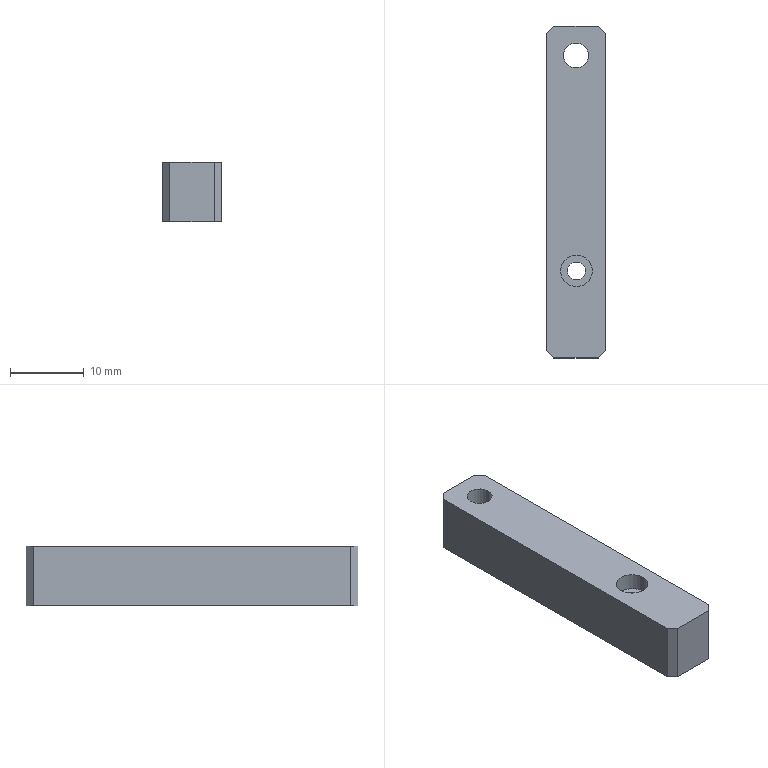Part | SolidWorks | features MirrorStock 1 | 1 solid | 23 faces | box 8 x 45 x 8 mm | volume 2651 mm3 | plane 13 | cylinder 10 | commonest cylinder face diameters 2.4 x2 3.4 x2 4 x2 4.3 x2 6 x2
STEP:
#1=CARTESIAN_POINT('',(-12.431,-38.2,-2.3));
#2=VERTEX_POINT('',#1);
#3=CARTESIAN_POINT('',(-8.131,-38.2,-2.3));
#4=VERTEX_POINT('',#3);
#5=CARTESIAN_POINT('',(-10.281,-38.2,-2.3));
#6=DIRECTION('',(0.,0.,-1.));
#7=DIRECTION('',(-1.,0.,0.));
#8=AXIS2_PLACEMENT_3D('',#5,#6,#7);
#9=CIRCLE('',#8,2.15);
#10=EDGE_CURVE('',#2,#4,#9,.T.);
#11=ORIENTED_EDGE('',*,*,#10,.T.);
#12=CARTESIAN_POINT('',(-8.131,-38.2,0.));
#13=VERTEX_POINT('',#12);
#14=CARTESIAN_POINT('',(-8.131,-38.2,0.));
#15=DIRECTION('',(0.,0.,1.));
#16=VECTOR('',#15,1000.);
#17=LINE('',#14,#16);
#18=EDGE_CURVE('',#4,#13,#17,.T.);
#19=ORIENTED_EDGE('',*,*,#18,.T.);
#20=CARTESIAN_POINT('',(-12.431,-38.2,0.));
#21=VERTEX_POINT('',#20);
#22=CARTESIAN_POINT('',(-10.281,-38.2,0.));
#23=DIRECTION('',(0.,0.,-1.));
#24=DIRECTION('',(-1.,0.,0.));
#25=AXIS2_PLACEMENT_3D('',#22,#23,#24);
#26=CIRCLE('',#25,2.15);
#27=EDGE_CURVE('',#21,#13,#26,.T.);
#28=ORIENTED_EDGE('',*,*,#27,.F.);
#29=CARTESIAN_POINT('',(-12.431,-38.2,0.));
#30=DIRECTION('',(0.,0.,1.));
#31=VECTOR('',#30,1000.);
#32=LINE('',#29,#31);
#33=EDGE_CURVE('',#2,#21,#32,.T.);
#34=ORIENTED_EDGE('',*,*,#33,.F.);
#35=EDGE_LOOP('',(#11,#19,#28,#34));
#36=FACE_OUTER_BOUND('',#35,.T.);
#37=CARTESIAN_POINT('',(-10.281,-38.2,0.));
#38=DIRECTION('',(0.,0.,1.));
#39=DIRECTION('',(-1.,0.,0.));
#40=AXIS2_PLACEMENT_3D('',#37,#38,#39);
#41=CYLINDRICAL_SURFACE('',#40,2.15);
#42=ADVANCED_FACE('',(#36),#41,.F.);
#43=CARTESIAN_POINT('',(-9.081,-38.2,-6.));
#44=VERTEX_POINT('',#43);
#45=CARTESIAN_POINT('',(-11.481,-38.2,-6.));
#46=VERTEX_POINT('',#45);
#47=CARTESIAN_POINT('',(-10.281,-38.2,-6.));
#48=DIRECTION('',(0.,0.,1.));
#49=DIRECTION('',(1.,0.,0.));
#50=AXIS2_PLACEMENT_3D('',#47,#48,#49);
#51=CIRCLE('',#50,1.2);
#52=EDGE_CURVE('',#44,#46,#51,.T.);
#53=ORIENTED_EDGE('',*,*,#52,.F.);
#54=CARTESIAN_POINT('',(-9.081,-38.2,-2.3));
#55=VERTEX_POINT('',#54);
#56=CARTESIAN_POINT('',(-9.081,-38.2,0.));
#57=DIRECTION('',(0.,0.,1.));
#58=VECTOR('',#57,1000.);
#59=LINE('',#56,#58);
#60=EDGE_CURVE('',#44,#55,#59,.T.);
#61=ORIENTED_EDGE('',*,*,#60,.T.);
#62=CARTESIAN_POINT('',(-11.481,-38.2,-2.3));
#63=VERTEX_POINT('',#62);
#64=CARTESIAN_POINT('',(-10.281,-38.2,-2.3));
#65=DIRECTION('',(0.,0.,-1.));
#66=DIRECTION('',(-1.,0.,0.));
#67=AXIS2_PLACEMENT_3D('',#64,#65,#66);
#68=CIRCLE('',#67,1.2);
#69=EDGE_CURVE('',#63,#55,#68,.T.);
#70=ORIENTED_EDGE('',*,*,#69,.F.);
#71=CARTESIAN_POINT('',(-11.481,-38.2,0.));
#72=DIRECTION('',(0.,0.,1.));
#73=VECTOR('',#72,1000.);
#74=LINE('',#71,#73);
#75=EDGE_CURVE('',#46,#63,#74,.T.);
#76=ORIENTED_EDGE('',*,*,#75,.F.);
#77=EDGE_LOOP('',(#53,#61,#70,#76));
#78=FACE_OUTER_BOUND('',#77,.T.);
#79=CARTESIAN_POINT('',(-10.281,-38.2,0.));
#80=DIRECTION('',(0.,0.,1.));
#81=DIRECTION('',(-1.,0.,0.));
#82=AXIS2_PLACEMENT_3D('',#79,#80,#81);
#83=CYLINDRICAL_SURFACE('',#82,1.2);
#84=ADVANCED_FACE('',(#78),#83,.F.);
#85=CARTESIAN_POINT('',(-8.281,-38.2,-6.));
#86=VERTEX_POINT('',#85);
#87=CARTESIAN_POINT('',(-12.281,-38.2,-6.));
#88=VERTEX_POINT('',#87);
#89=CARTESIAN_POINT('',(-10.281,-38.2,-6.));
#90=DIRECTION('',(0.,0.,1.));
#91=DIRECTION('',(1.,0.,0.));
#92=AXIS2_PLACEMENT_3D('',#89,#90,#91);
#93=CIRCLE('',#92,2.);
#94=EDGE_CURVE('',#86,#88,#93,.T.);
#95=ORIENTED_EDGE('',*,*,#94,.T.);
#96=CARTESIAN_POINT('',(-12.281,-38.2,-8.));
#97=VERTEX_POINT('',#96);
#98=CARTESIAN_POINT('',(-12.281,-38.2,-6.));
#99=DIRECTION('',(0.,0.,-1.));
#100=VECTOR('',#99,1000.);
#101=LINE('',#98,#100);
#102=EDGE_CURVE('',#88,#97,#101,.T.);
#103=ORIENTED_EDGE('',*,*,#102,.T.);
#104=CARTESIAN_POINT('',(-8.281,-38.2,-8.));
#105=VERTEX_POINT('',#104);
#106=CARTESIAN_POINT('',(-10.281,-38.2,-8.));
#107=DIRECTION('',(0.,0.,1.));
#108=DIRECTION('',(1.,0.,0.));
#109=AXIS2_PLACEMENT_3D('',#106,#107,#108);
#110=CIRCLE('',#109,2.);
#111=EDGE_CURVE('',#105,#97,#110,.T.);
#112=ORIENTED_EDGE('',*,*,#111,.F.);
#113=CARTESIAN_POINT('',(-8.281,-38.2,-6.));
#114=DIRECTION('',(0.,0.,-1.));
#115=VECTOR('',#114,1000.);
#116=LINE('',#113,#115);
#117=EDGE_CURVE('',#86,#105,#116,.T.);
#118=ORIENTED_EDGE('',*,*,#117,.F.);
#119=EDGE_LOOP('',(#95,#103,#112,#118));
#120=FACE_OUTER_BOUND('',#119,.T.);
#121=CARTESIAN_POINT('',(-10.281,-38.2,-6.));
#122=DIRECTION('',(0.,0.,-1.));
#123=DIRECTION('',(1.,0.,0.));
#124=AXIS2_PLACEMENT_3D('',#121,#122,#123);
#125=CYLINDRICAL_SURFACE('',#124,2.);
#126=ADVANCED_FACE('',(#120),#125,.F.);
#127=CARTESIAN_POINT('',(-7.345,-9.,-4.6));
#128=VERTEX_POINT('',#127);
#129=CARTESIAN_POINT('',(-13.345,-9.,-4.6));
#130=VERTEX_POINT('',#129);
#131=CARTESIAN_POINT('',(-10.345,-9.,-4.6));
#132=DIRECTION('',(0.,0.,1.));
#133=DIRECTION('',(1.,0.,0.));
#134=AXIS2_PLACEMENT_3D('',#131,#132,#133);
#135=CIRCLE('',#134,3.);
#136=EDGE_CURVE('',#128,#130,#135,.T.);
#137=ORIENTED_EDGE('',*,*,#136,.T.);
#138=CARTESIAN_POINT('',(-13.345,-9.,-8.));
#139=VERTEX_POINT('',#138);
#140=CARTESIAN_POINT('',(-13.345,-9.,-8.));
#141=DIRECTION('',(0.,0.,-1.));
#142=VECTOR('',#141,1000.);
#143=LINE('',#140,#142);
#144=EDGE_CURVE('',#130,#139,#143,.T.);
#145=ORIENTED_EDGE('',*,*,#144,.T.);
#146=CARTESIAN_POINT('',(-7.345,-9.,-8.));
#147=VERTEX_POINT('',#146);
#148=CARTESIAN_POINT('',(-10.345,-9.,-8.));
#149=DIRECTION('',(0.,0.,1.));
#150=DIRECTION('',(1.,0.,0.));
#151=AXIS2_PLACEMENT_3D('',#148,#149,#150);
#152=CIRCLE('',#151,3.);
#153=EDGE_CURVE('',#147,#139,#152,.T.);
#154=ORIENTED_EDGE('',*,*,#153,.F.);
#155=CARTESIAN_POINT('',(-7.345,-9.,-8.));
#156=DIRECTION('',(0.,0.,-1.));
#157=VECTOR('',#156,1000.);
#158=LINE('',#155,#157);
#159=EDGE_CURVE('',#128,#147,#158,.T.);
#160=ORIENTED_EDGE('',*,*,#159,.F.);
#161=EDGE_LOOP('',(#137,#145,#154,#160));
#162=FACE_OUTER_BOUND('',#161,.T.);
#163=CARTESIAN_POINT('',(-10.345,-9.,-8.));
#164=DIRECTION('',(0.,0.,-1.));
#165=DIRECTION('',(1.,0.,0.));
#166=AXIS2_PLACEMENT_3D('',#163,#164,#165);
#167=CYLINDRICAL_SURFACE('',#166,3.);
#168=ADVANCED_FACE('',(#162),#167,.F.);
#169=CARTESIAN_POINT('',(-8.645,-9.,0.));
#170=VERTEX_POINT('',#169);
#171=CARTESIAN_POINT('',(-12.045,-9.,0.));
#172=VERTEX_POINT('',#171);
#173=CARTESIAN_POINT('',(-10.345,-9.,0.));
#174=DIRECTION('',(0.,0.,1.));
#175=DIRECTION('',(1.,0.,0.));
#176=AXIS2_PLACEMENT_3D('',#173,#174,#175);
#177=CIRCLE('',#176,1.7);
#178=EDGE_CURVE('',#170,#172,#177,.T.);
#179=ORIENTED_EDGE('',*,*,#178,.T.);
#180=CARTESIAN_POINT('',(-12.045,-9.,-4.6));
#181=VERTEX_POINT('',#180);
#182=CARTESIAN_POINT('',(-12.045,-9.,-8.));
#183=DIRECTION('',(0.,0.,-1.));
#184=VECTOR('',#183,1000.);
#185=LINE('',#182,#184);
#186=EDGE_CURVE('',#172,#181,#185,.T.);
#187=ORIENTED_EDGE('',*,*,#186,.T.);
#188=CARTESIAN_POINT('',(-8.645,-9.,-4.6));
#189=VERTEX_POINT('',#188);
#190=CARTESIAN_POINT('',(-10.345,-9.,-4.6));
#191=DIRECTION('',(0.,0.,1.));
#192=DIRECTION('',(1.,0.,0.));
#193=AXIS2_PLACEMENT_3D('',#190,#191,#192);
#194=CIRCLE('',#193,1.7);
#195=EDGE_CURVE('',#189,#181,#194,.T.);
#196=ORIENTED_EDGE('',*,*,#195,.F.);
#197=CARTESIAN_POINT('',(-8.645,-9.,-8.));
#198=DIRECTION('',(0.,0.,-1.));
#199=VECTOR('',#198,1000.);
#200=LINE('',#197,#199);
#201=EDGE_CURVE('',#170,#189,#200,.T.);
#202=ORIENTED_EDGE('',*,*,#201,.F.);
#203=EDGE_LOOP('',(#179,#187,#196,#202));
#204=FACE_OUTER_BOUND('',#203,.T.);
#205=CARTESIAN_POINT('',(-10.345,-9.,-8.));
#206=DIRECTION('',(0.,0.,-1.));
#207=DIRECTION('',(1.,0.,0.));
#208=AXIS2_PLACEMENT_3D('',#205,#206,#207);
#209=CYLINDRICAL_SURFACE('',#208,1.7);
#210=ADVANCED_FACE('',(#204),#209,.F.);
#211=CARTESIAN_POINT('',(-13.345,-5.,-8.));
#212=VERTEX_POINT('',#211);
#213=CARTESIAN_POINT('',(-7.345,-5.,-8.));
#214=VERTEX_POINT('',#213);
#215=CARTESIAN_POINT('',(-14.345,-5.,-8.));
#216=DIRECTION('',(1.,0.,0.));
#217=VECTOR('',#216,1000.);
#218=LINE('',#215,#217);
#219=EDGE_CURVE('',#212,#214,#218,.T.);
#220=ORIENTED_EDGE('',*,*,#219,.F.);
#221=CARTESIAN_POINT('',(-13.345,-5.,0.));
#222=VERTEX_POINT('',#221);
#223=CARTESIAN_POINT('',(-13.345,-5.,-8.));
#224=DIRECTION('',(0.,0.,-1.));
#225=VECTOR('',#224,1000.);
#226=LINE('',#223,#225);
#227=EDGE_CURVE('',#222,#212,#226,.T.);
#228=ORIENTED_EDGE('',*,*,#227,.F.);
#229=CARTESIAN_POINT('',(-7.345,-5.,0.));
#230=VERTEX_POINT('',#229);
#231=CARTESIAN_POINT('',(-14.345,-5.,0.));
#232=DIRECTION('',(1.,0.,0.));
#233=VECTOR('',#232,1000.);
#234=LINE('',#231,#233);
#235=EDGE_CURVE('',#222,#230,#234,.T.);
#236=ORIENTED_EDGE('',*,*,#235,.T.);
#237=CARTESIAN_POINT('',(-7.345,-5.,-8.));
#238=DIRECTION('',(0.,0.,1.));
#239=VECTOR('',#238,1000.);
#240=LINE('',#237,#239);
#241=EDGE_CURVE('',#214,#230,#240,.T.);
#242=ORIENTED_EDGE('',*,*,#241,.F.);
#243=EDGE_LOOP('',(#220,#228,#236,#242));
#244=FACE_OUTER_BOUND('',#243,.T.);
#245=CARTESIAN_POINT('',(-14.345,-5.,-8.));
#246=DIRECTION('',(0.,1.,0.));
#247=DIRECTION('',(0.,0.,-1.));
#248=AXIS2_PLACEMENT_3D('',#245,#246,#247);
#249=PLANE('',#248);
#250=ADVANCED_FACE('',(#244),#249,.T.);
#251=CARTESIAN_POINT('',(-14.345,-6.,0.));
#252=VERTEX_POINT('',#251);
#253=CARTESIAN_POINT('',(-14.345,-49.,0.));
#254=VERTEX_POINT('',#253);
#255=CARTESIAN_POINT('',(-14.345,-5.,0.));
#256=DIRECTION('',(0.,-1.,0.));
#257=VECTOR('',#256,1000.);
#258=LINE('',#255,#257);
#259=EDGE_CURVE('',#252,#254,#258,.T.);
#260=ORIENTED_EDGE('',*,*,#259,.F.);
#261=CARTESIAN_POINT('',(-14.345,-6.,-8.));
#262=VERTEX_POINT('',#261);
#263=CARTESIAN_POINT('',(-14.345,-6.,0.));
#264=DIRECTION('',(0.,0.,1.));
#265=VECTOR('',#264,1000.);
#266=LINE('',#263,#265);
#267=EDGE_CURVE('',#262,#252,#266,.T.);
#268=ORIENTED_EDGE('',*,*,#267,.F.);
#269=CARTESIAN_POINT('',(-14.345,-49.,-8.));
#270=VERTEX_POINT('',#269);
#271=CARTESIAN_POINT('',(-14.345,-5.,-8.));
#272=DIRECTION('',(0.,-1.,0.));
#273=VECTOR('',#272,1000.);
#274=LINE('',#271,#273);
#275=EDGE_CURVE('',#262,#270,#274,.T.);
#276=ORIENTED_EDGE('',*,*,#275,.T.);
#277=CARTESIAN_POINT('',(-14.345,-49.,-8.));
#278=DIRECTION('',(0.,0.,-1.));
#279=VECTOR('',#278,1000.);
#280=LINE('',#277,#279);
#281=EDGE_CURVE('',#254,#270,#280,.T.);
#282=ORIENTED_EDGE('',*,*,#281,.F.);
#283=EDGE_LOOP('',(#260,#268,#276,#282));
#284=FACE_OUTER_BOUND('',#283,.T.);
#285=CARTESIAN_POINT('',(-14.345,-5.,-8.));
#286=DIRECTION('',(1.,0.,0.));
#287=DIRECTION('',(0.,1.,0.));
#288=AXIS2_PLACEMENT_3D('',#285,#286,#287);
#289=PLANE('',#288);
#290=ADVANCED_FACE('',(#284),#289,.F.);
#291=CARTESIAN_POINT('',(-13.345,-50.,0.));
#292=VERTEX_POINT('',#291);
#293=CARTESIAN_POINT('',(-7.345,-50.,0.));
#294=VERTEX_POINT('',#293);
#295=CARTESIAN_POINT('',(-14.345,-50.,0.));
#296=DIRECTION('',(1.,0.,0.));
#297=VECTOR('',#296,1000.);
#298=LINE('',#295,#297);
#299=EDGE_CURVE('',#292,#294,#298,.T.);
#300=ORIENTED_EDGE('',*,*,#299,.F.);
#301=CARTESIAN_POINT('',(-13.345,-50.,-8.));
#302=VERTEX_POINT('',#301);
#303=CARTESIAN_POINT('',(-13.345,-50.,-8.));
#304=DIRECTION('',(0.,0.,1.));
#305=VECTOR('',#304,1000.);
#306=LINE('',#303,#305);
#307=EDGE_CURVE('',#302,#292,#306,.T.);
#308=ORIENTED_EDGE('',*,*,#307,.F.);
#309=CARTESIAN_POINT('',(-7.345,-50.,-8.));
#310=VERTEX_POINT('',#309);
#311=CARTESIAN_POINT('',(-14.345,-50.,-8.));
#312=DIRECTION('',(1.,0.,0.));
#313=VECTOR('',#312,1000.);
#314=LINE('',#311,#313);
#315=EDGE_CURVE('',#302,#310,#314,.T.);
#316=ORIENTED_EDGE('',*,*,#315,.T.);
#317=CARTESIAN_POINT('',(-7.345,-50.,-8.));
#318=DIRECTION('',(0.,0.,-1.));
#319=VECTOR('',#318,1000.);
#320=LINE('',#317,#319);
#321=EDGE_CURVE('',#294,#310,#320,.T.);
#322=ORIENTED_EDGE('',*,*,#321,.F.);
#323=EDGE_LOOP('',(#300,#308,#316,#322));
#324=FACE_OUTER_BOUND('',#323,.T.);
#325=CARTESIAN_POINT('',(-14.345,-50.,-8.));
#326=DIRECTION('',(0.,1.,0.));
#327=DIRECTION('',(0.,0.,-1.));
#328=AXIS2_PLACEMENT_3D('',#325,#326,#327);
#329=PLANE('',#328);
#330=ADVANCED_FACE('',(#324),#329,.F.);
#331=CARTESIAN_POINT('',(-6.345,-6.,-8.));
#332=VERTEX_POINT('',#331);
#333=CARTESIAN_POINT('',(-6.345,-49.,-8.));
#334=VERTEX_POINT('',#333);
#335=CARTESIAN_POINT('',(-6.345,-5.,-8.));
#336=DIRECTION('',(0.,-1.,0.));
#337=VECTOR('',#336,1000.);
#338=LINE('',#335,#337);
#339=EDGE_CURVE('',#332,#334,#338,.T.);
#340=ORIENTED_EDGE('',*,*,#339,.F.);
#341=CARTESIAN_POINT('',(-6.345,-6.,0.));
#342=VERTEX_POINT('',#341);
#343=CARTESIAN_POINT('',(-6.345,-6.,-8.));
#344=DIRECTION('',(0.,0.,-1.));
#345=VECTOR('',#344,1000.);
#346=LINE('',#343,#345);
#347=EDGE_CURVE('',#342,#332,#346,.T.);
#348=ORIENTED_EDGE('',*,*,#347,.F.);
#349=CARTESIAN_POINT('',(-6.345,-49.,0.));
#350=VERTEX_POINT('',#349);
#351=CARTESIAN_POINT('',(-6.345,-5.,0.));
#352=DIRECTION('',(0.,-1.,0.));
#353=VECTOR('',#352,1000.);
#354=LINE('',#351,#353);
#355=EDGE_CURVE('',#342,#350,#354,.T.);
#356=ORIENTED_EDGE('',*,*,#355,.T.);
#357=CARTESIAN_POINT('',(-6.345,-49.,0.));
#358=DIRECTION('',(0.,0.,1.));
#359=VECTOR('',#358,1000.);
#360=LINE('',#357,#359);
#361=EDGE_CURVE('',#334,#350,#360,.T.);
#362=ORIENTED_EDGE('',*,*,#361,.F.);
#363=EDGE_LOOP('',(#340,#348,#356,#362));
#364=FACE_OUTER_BOUND('',#363,.T.);
#365=CARTESIAN_POINT('',(-6.345,-5.,-8.));
#366=DIRECTION('',(1.,0.,0.));
#367=DIRECTION('',(0.,1.,0.));
#368=AXIS2_PLACEMENT_3D('',#365,#366,#367);
#369=PLANE('',#368);
#370=ADVANCED_FACE('',(#364),#369,.T.);
#371=ORIENTED_EDGE('',*,*,#111,.T.);
#372=CARTESIAN_POINT('',(-10.281,-38.2,-8.));
#373=DIRECTION('',(0.,0.,1.));
#374=DIRECTION('',(1.,0.,0.));
#375=AXIS2_PLACEMENT_3D('',#372,#373,#374);
#376=CIRCLE('',#375,2.);
#377=EDGE_CURVE('',#97,#105,#376,.T.);
#378=ORIENTED_EDGE('',*,*,#377,.T.);
#379=EDGE_LOOP('',(#371,#378));
#380=FACE_BOUND('',#379,.T.);
#381=ORIENTED_EDGE('',*,*,#153,.T.);
#382=CARTESIAN_POINT('',(-10.345,-9.,-8.));
#383=DIRECTION('',(0.,0.,1.));
#384=DIRECTION('',(1.,0.,0.));
#385=AXIS2_PLACEMENT_3D('',#382,#383,#384);
#386=CIRCLE('',#385,3.);
#387=EDGE_CURVE('',#139,#147,#386,.T.);
#388=ORIENTED_EDGE('',*,*,#387,.T.);
#389=EDGE_LOOP('',(#381,#388));
#390=FACE_BOUND('',#389,.T.);
#391=ORIENTED_EDGE('',*,*,#315,.F.);
#392=CARTESIAN_POINT('',(-13.345,-50.,-8.));
#393=DIRECTION('',(0.7071,-0.7071,0.));
#394=VECTOR('',#393,1000.);
#395=LINE('',#392,#394);
#396=EDGE_CURVE('',#270,#302,#395,.T.);
#397=ORIENTED_EDGE('',*,*,#396,.F.);
#398=ORIENTED_EDGE('',*,*,#275,.F.);
#399=CARTESIAN_POINT('',(-14.345,-6.,-8.));
#400=DIRECTION('',(-0.7071,-0.7071,0.));
#401=VECTOR('',#400,1000.);
#402=LINE('',#399,#401);
#403=EDGE_CURVE('',#212,#262,#402,.T.);
#404=ORIENTED_EDGE('',*,*,#403,.F.);
#405=ORIENTED_EDGE('',*,*,#219,.T.);
#406=CARTESIAN_POINT('',(-7.345,-5.,-8.));
#407=DIRECTION('',(-0.7071,0.7071,0.));
#408=VECTOR('',#407,1000.);
#409=LINE('',#406,#408);
#410=EDGE_CURVE('',#332,#214,#409,.T.);
#411=ORIENTED_EDGE('',*,*,#410,.F.);
#412=ORIENTED_EDGE('',*,*,#339,.T.);
#413=CARTESIAN_POINT('',(-6.345,-49.,-8.));
#414=DIRECTION('',(0.7071,0.7071,0.));
#415=VECTOR('',#414,1000.);
#416=LINE('',#413,#415);
#417=EDGE_CURVE('',#310,#334,#416,.T.);
#418=ORIENTED_EDGE('',*,*,#417,.F.);
#419=EDGE_LOOP('',(#391,#397,#398,#404,#405,#411,#412,#418));
#420=FACE_OUTER_BOUND('',#419,.T.);
#421=CARTESIAN_POINT('',(0.,0.,-8.));
#422=DIRECTION('',(0.,0.,1.));
#423=DIRECTION('',(-1.,0.,0.));
#424=AXIS2_PLACEMENT_3D('',#421,#422,#423);
#425=PLANE('',#424);
#426=ADVANCED_FACE('',(#380,#390,#420),#425,.F.);
#427=ORIENTED_EDGE('',*,*,#27,.T.);
#428=CARTESIAN_POINT('',(-10.281,-38.2,0.));
#429=DIRECTION('',(0.,0.,-1.));
#430=DIRECTION('',(-1.,0.,0.));
#431=AXIS2_PLACEMENT_3D('',#428,#429,#430);
#432=CIRCLE('',#431,2.15);
#433=EDGE_CURVE('',#13,#21,#432,.T.);
#434=ORIENTED_EDGE('',*,*,#433,.T.);
#435=EDGE_LOOP('',(#427,#434));
#436=FACE_BOUND('',#435,.T.);
#437=ORIENTED_EDGE('',*,*,#178,.F.);
#438=CARTESIAN_POINT('',(-10.345,-9.,0.));
#439=DIRECTION('',(0.,0.,1.));
#440=DIRECTION('',(1.,0.,0.));
#441=AXIS2_PLACEMENT_3D('',#438,#439,#440);
#442=CIRCLE('',#441,1.7);
#443=EDGE_CURVE('',#172,#170,#442,.T.);
#444=ORIENTED_EDGE('',*,*,#443,.F.);
#445=EDGE_LOOP('',(#437,#444));
#446=FACE_BOUND('',#445,.T.);
#447=ORIENTED_EDGE('',*,*,#355,.F.);
#448=CARTESIAN_POINT('',(-6.172,-6.172,0.));
#449=DIRECTION('',(0.7071,-0.7071,0.));
#450=VECTOR('',#449,1000.);
#451=LINE('',#448,#450);
#452=EDGE_CURVE('',#230,#342,#451,.T.);
#453=ORIENTED_EDGE('',*,*,#452,.F.);
#454=ORIENTED_EDGE('',*,*,#235,.F.);
#455=CARTESIAN_POINT('',(-4.172,4.172,0.));
#456=DIRECTION('',(0.7071,0.7071,0.));
#457=VECTOR('',#456,1000.);
#458=LINE('',#455,#457);
#459=EDGE_CURVE('',#252,#222,#458,.T.);
#460=ORIENTED_EDGE('',*,*,#459,.F.);
#461=ORIENTED_EDGE('',*,*,#259,.T.);
#462=CARTESIAN_POINT('',(-31.672,-31.672,0.));
#463=DIRECTION('',(-0.7071,0.7071,0.));
#464=VECTOR('',#463,1000.);
#465=LINE('',#462,#464);
#466=EDGE_CURVE('',#292,#254,#465,.T.);
#467=ORIENTED_EDGE('',*,*,#466,.F.);
#468=ORIENTED_EDGE('',*,*,#299,.T.);
#469=CARTESIAN_POINT('',(21.328,-21.328,0.));
#470=DIRECTION('',(-0.7071,-0.7071,0.));
#471=VECTOR('',#470,1000.);
#472=LINE('',#469,#471);
#473=EDGE_CURVE('',#350,#294,#472,.T.);
#474=ORIENTED_EDGE('',*,*,#473,.F.);
#475=EDGE_LOOP('',(#447,#453,#454,#460,#461,#467,#468,#474));
#476=FACE_OUTER_BOUND('',#475,.T.);
#477=CARTESIAN_POINT('',(0.,0.,0.));
#478=DIRECTION('',(0.,0.,1.));
#479=DIRECTION('',(-1.,0.,0.));
#480=AXIS2_PLACEMENT_3D('',#477,#478,#479);
#481=PLANE('',#480);
#482=ADVANCED_FACE('',(#436,#446,#476),#481,.T.);
#483=ORIENTED_EDGE('',*,*,#186,.F.);
#484=ORIENTED_EDGE('',*,*,#443,.T.);
#485=ORIENTED_EDGE('',*,*,#201,.T.);
#486=CARTESIAN_POINT('',(-10.345,-9.,-4.6));
#487=DIRECTION('',(0.,0.,1.));
#488=DIRECTION('',(1.,0.,0.));
#489=AXIS2_PLACEMENT_3D('',#486,#487,#488);
#490=CIRCLE('',#489,1.7);
#491=EDGE_CURVE('',#181,#189,#490,.T.);
#492=ORIENTED_EDGE('',*,*,#491,.F.);
#493=EDGE_LOOP('',(#483,#484,#485,#492));
#494=FACE_OUTER_BOUND('',#493,.T.);
#495=CARTESIAN_POINT('',(-10.345,-9.,-8.));
#496=DIRECTION('',(0.,0.,-1.));
#497=DIRECTION('',(1.,0.,0.));
#498=AXIS2_PLACEMENT_3D('',#495,#496,#497);
#499=CYLINDRICAL_SURFACE('',#498,1.7);
#500=ADVANCED_FACE('',(#494),#499,.F.);
#501=ORIENTED_EDGE('',*,*,#195,.T.);
#502=ORIENTED_EDGE('',*,*,#491,.T.);
#503=EDGE_LOOP('',(#501,#502));
#504=FACE_BOUND('',#503,.T.);
#505=ORIENTED_EDGE('',*,*,#136,.F.);
#506=CARTESIAN_POINT('',(-10.345,-9.,-4.6));
#507=DIRECTION('',(0.,0.,1.));
#508=DIRECTION('',(1.,0.,0.));
#509=AXIS2_PLACEMENT_3D('',#506,#507,#508);
#510=CIRCLE('',#509,3.);
#511=EDGE_CURVE('',#130,#128,#510,.T.);
#512=ORIENTED_EDGE('',*,*,#511,.F.);
#513=EDGE_LOOP('',(#505,#512));
#514=FACE_OUTER_BOUND('',#513,.T.);
#515=CARTESIAN_POINT('',(-8.645,-9.,-4.6));
#516=DIRECTION('',(0.,0.,1.));
#517=DIRECTION('',(-1.,0.,0.));
#518=AXIS2_PLACEMENT_3D('',#515,#516,#517);
#519=PLANE('',#518);
#520=ADVANCED_FACE('',(#504,#514),#519,.F.);
#521=ORIENTED_EDGE('',*,*,#144,.F.);
#522=ORIENTED_EDGE('',*,*,#511,.T.);
#523=ORIENTED_EDGE('',*,*,#159,.T.);
#524=ORIENTED_EDGE('',*,*,#387,.F.);
#525=EDGE_LOOP('',(#521,#522,#523,#524));
#526=FACE_OUTER_BOUND('',#525,.T.);
#527=CARTESIAN_POINT('',(-10.345,-9.,-8.));
#528=DIRECTION('',(0.,0.,-1.));
#529=DIRECTION('',(1.,0.,0.));
#530=AXIS2_PLACEMENT_3D('',#527,#528,#529);
#531=CYLINDRICAL_SURFACE('',#530,3.);
#532=ADVANCED_FACE('',(#526),#531,.F.);
#533=ORIENTED_EDGE('',*,*,#102,.F.);
#534=CARTESIAN_POINT('',(-10.281,-38.2,-6.));
#535=DIRECTION('',(0.,0.,1.));
#536=DIRECTION('',(1.,0.,0.));
#537=AXIS2_PLACEMENT_3D('',#534,#535,#536);
#538=CIRCLE('',#537,2.);
#539=EDGE_CURVE('',#88,#86,#538,.T.);
#540=ORIENTED_EDGE('',*,*,#539,.T.);
#541=ORIENTED_EDGE('',*,*,#117,.T.);
#542=ORIENTED_EDGE('',*,*,#377,.F.);
#543=EDGE_LOOP('',(#533,#540,#541,#542));
#544=FACE_OUTER_BOUND('',#543,.T.);
#545=CARTESIAN_POINT('',(-10.281,-38.2,-6.));
#546=DIRECTION('',(0.,0.,-1.));
#547=DIRECTION('',(1.,0.,0.));
#548=AXIS2_PLACEMENT_3D('',#545,#546,#547);
#549=CYLINDRICAL_SURFACE('',#548,2.);
#550=ADVANCED_FACE('',(#544),#549,.F.);
#551=CARTESIAN_POINT('',(-10.281,-38.2,-6.));
#552=DIRECTION('',(0.,0.,1.));
#553=DIRECTION('',(1.,0.,0.));
#554=AXIS2_PLACEMENT_3D('',#551,#552,#553);
#555=CIRCLE('',#554,1.2);
#556=EDGE_CURVE('',#46,#44,#555,.T.);
#557=ORIENTED_EDGE('',*,*,#556,.T.);
#558=ORIENTED_EDGE('',*,*,#52,.T.);
#559=EDGE_LOOP('',(#557,#558));
#560=FACE_BOUND('',#559,.T.);
#561=ORIENTED_EDGE('',*,*,#94,.F.);
#562=ORIENTED_EDGE('',*,*,#539,.F.);
#563=EDGE_LOOP('',(#561,#562));
#564=FACE_OUTER_BOUND('',#563,.T.);
#565=CARTESIAN_POINT('',(-10.281,-38.2,-6.));
#566=DIRECTION('',(0.,0.,-1.));
#567=DIRECTION('',(1.,0.,0.));
#568=AXIS2_PLACEMENT_3D('',#565,#566,#567);
#569=PLANE('',#568);
#570=ADVANCED_FACE('',(#560,#564),#569,.T.);
#571=ORIENTED_EDGE('',*,*,#60,.F.);
#572=ORIENTED_EDGE('',*,*,#556,.F.);
#573=ORIENTED_EDGE('',*,*,#75,.T.);
#574=CARTESIAN_POINT('',(-10.281,-38.2,-2.3));
#575=DIRECTION('',(0.,0.,-1.));
#576=DIRECTION('',(-1.,0.,0.));
#577=AXIS2_PLACEMENT_3D('',#574,#575,#576);
#578=CIRCLE('',#577,1.2);
#579=EDGE_CURVE('',#55,#63,#578,.T.);
#580=ORIENTED_EDGE('',*,*,#579,.F.);
#581=EDGE_LOOP('',(#571,#572,#573,#580));
#582=FACE_OUTER_BOUND('',#581,.T.);
#583=CARTESIAN_POINT('',(-10.281,-38.2,0.));
#584=DIRECTION('',(0.,0.,1.));
#585=DIRECTION('',(-1.,0.,0.));
#586=AXIS2_PLACEMENT_3D('',#583,#584,#585);
#587=CYLINDRICAL_SURFACE('',#586,1.2);
#588=ADVANCED_FACE('',(#582),#587,.F.);
#589=ORIENTED_EDGE('',*,*,#69,.T.);
#590=ORIENTED_EDGE('',*,*,#579,.T.);
#591=EDGE_LOOP('',(#589,#590));
#592=FACE_BOUND('',#591,.T.);
#593=ORIENTED_EDGE('',*,*,#10,.F.);
#594=CARTESIAN_POINT('',(-10.281,-38.2,-2.3));
#595=DIRECTION('',(0.,0.,-1.));
#596=DIRECTION('',(-1.,0.,0.));
#597=AXIS2_PLACEMENT_3D('',#594,#595,#596);
#598=CIRCLE('',#597,2.15);
#599=EDGE_CURVE('',#4,#2,#598,.T.);
#600=ORIENTED_EDGE('',*,*,#599,.F.);
#601=EDGE_LOOP('',(#593,#600));
#602=FACE_OUTER_BOUND('',#601,.T.);
#603=CARTESIAN_POINT('',(-9.081,-38.2,-2.3));
#604=DIRECTION('',(0.,0.,-1.));
#605=DIRECTION('',(1.,0.,0.));
#606=AXIS2_PLACEMENT_3D('',#603,#604,#605);
#607=PLANE('',#606);
#608=ADVANCED_FACE('',(#592,#602),#607,.F.);
#609=ORIENTED_EDGE('',*,*,#18,.F.);
#610=ORIENTED_EDGE('',*,*,#599,.T.);
#611=ORIENTED_EDGE('',*,*,#33,.T.);
#612=ORIENTED_EDGE('',*,*,#433,.F.);
#613=EDGE_LOOP('',(#609,#610,#611,#612));
#614=FACE_OUTER_BOUND('',#613,.T.);
#615=CARTESIAN_POINT('',(-10.281,-38.2,0.));
#616=DIRECTION('',(0.,0.,1.));
#617=DIRECTION('',(-1.,0.,0.));
#618=AXIS2_PLACEMENT_3D('',#615,#616,#617);
#619=CYLINDRICAL_SURFACE('',#618,2.15);
#620=ADVANCED_FACE('',(#614),#619,.F.);
#621=ORIENTED_EDGE('',*,*,#417,.T.);
#622=ORIENTED_EDGE('',*,*,#361,.T.);
#623=ORIENTED_EDGE('',*,*,#473,.T.);
#624=ORIENTED_EDGE('',*,*,#321,.T.);
#625=EDGE_LOOP('',(#621,#622,#623,#624));
#626=FACE_OUTER_BOUND('',#625,.T.);
#627=CARTESIAN_POINT('',(-6.345,-49.,-8.));
#628=DIRECTION('',(0.7071,-0.7071,0.));
#629=DIRECTION('',(0.,0.,-1.));
#630=AXIS2_PLACEMENT_3D('',#627,#628,#629);
#631=PLANE('',#630);
#632=ADVANCED_FACE('',(#626),#631,.T.);
#633=ORIENTED_EDGE('',*,*,#396,.T.);
#634=ORIENTED_EDGE('',*,*,#307,.T.);
#635=ORIENTED_EDGE('',*,*,#466,.T.);
#636=ORIENTED_EDGE('',*,*,#281,.T.);
#637=EDGE_LOOP('',(#633,#634,#635,#636));
#638=FACE_OUTER_BOUND('',#637,.T.);
#639=CARTESIAN_POINT('',(-13.345,-50.,-8.));
#640=DIRECTION('',(0.7071,0.7071,0.));
#641=DIRECTION('',(0.,0.,1.));
#642=AXIS2_PLACEMENT_3D('',#639,#640,#641);
#643=PLANE('',#642);
#644=ADVANCED_FACE('',(#638),#643,.F.);
#645=ORIENTED_EDGE('',*,*,#410,.T.);
#646=ORIENTED_EDGE('',*,*,#241,.T.);
#647=ORIENTED_EDGE('',*,*,#452,.T.);
#648=ORIENTED_EDGE('',*,*,#347,.T.);
#649=EDGE_LOOP('',(#645,#646,#647,#648));
#650=FACE_OUTER_BOUND('',#649,.T.);
#651=CARTESIAN_POINT('',(-7.345,-5.,-8.));
#652=DIRECTION('',(-0.7071,-0.7071,0.));
#653=DIRECTION('',(0.,0.,1.));
#654=AXIS2_PLACEMENT_3D('',#651,#652,#653);
#655=PLANE('',#654);
#656=ADVANCED_FACE('',(#650),#655,.F.);
#657=ORIENTED_EDGE('',*,*,#403,.T.);
#658=ORIENTED_EDGE('',*,*,#267,.T.);
#659=ORIENTED_EDGE('',*,*,#459,.T.);
#660=ORIENTED_EDGE('',*,*,#227,.T.);
#661=EDGE_LOOP('',(#657,#658,#659,#660));
#662=FACE_OUTER_BOUND('',#661,.T.);
#663=CARTESIAN_POINT('',(-14.345,-6.,-8.));
#664=DIRECTION('',(-0.7071,0.7071,0.));
#665=DIRECTION('',(0.,0.,-1.));
#666=AXIS2_PLACEMENT_3D('',#663,#664,#665);
#667=PLANE('',#666);
#668=ADVANCED_FACE('',(#662),#667,.T.);
#669=CLOSED_SHELL('',(#42,#84,#126,#168,#210,#250,#290,#330,#370,#426,#482,#500,#520,#532,#550,#570,#588,#608,#620,#632,#644,#656,#668));
#670=MANIFOLD_SOLID_BREP('',#669);
#671=CARTESIAN_POINT('',(0.,0.,0.));
#672=DIRECTION('',(0.,0.,1.));
#673=DIRECTION('',(1.,0.,0.));
#674=AXIS2_PLACEMENT_3D('',#671,#672,#673);
#675=(LENGTH_UNIT()NAMED_UNIT(*)SI_UNIT(.MILLI.,.METRE.));
#676=UNCERTAINTY_MEASURE_WITH_UNIT(LENGTH_MEASURE(0.00001),#675,'','');
#677=(NAMED_UNIT(*)PLANE_ANGLE_UNIT()SI_UNIT($,.RADIAN.));
#678=(NAMED_UNIT(*)SI_UNIT($,.STERADIAN.)SOLID_ANGLE_UNIT());
#679=(GEOMETRIC_REPRESENTATION_CONTEXT(3)GLOBAL_UNCERTAINTY_ASSIGNED_CONTEXT((#676))GLOBAL_UNIT_ASSIGNED_CONTEXT((#675,#677,#678))REPRESENTATION_CONTEXT('',''));
#680=ADVANCED_BREP_SHAPE_REPRESENTATION('',(#670,#674),#679);